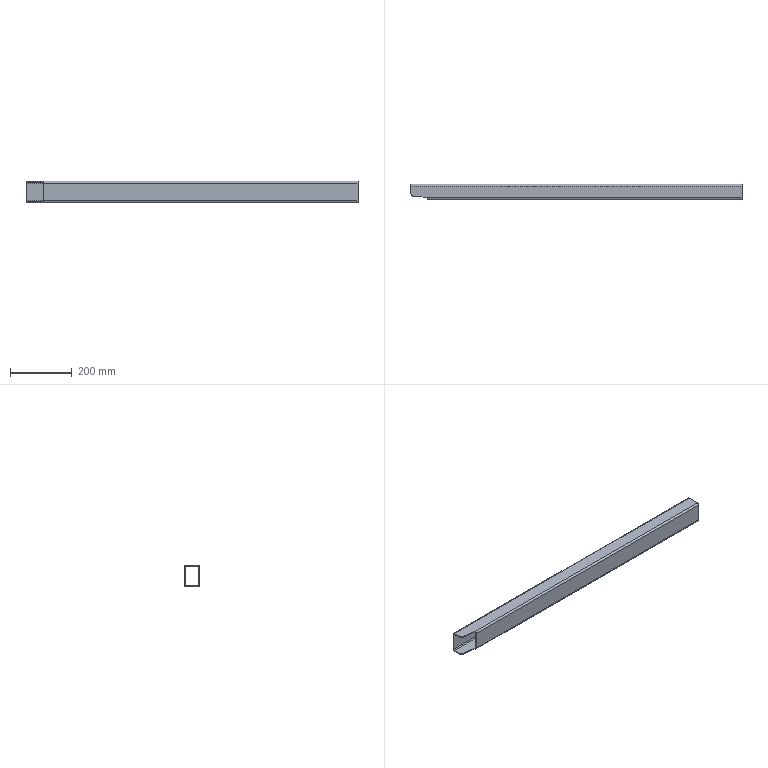Part | SolidWorks | 1 solid | 25 faces | box 1074 x 50 x 70 mm | volume 695582 mm3 | plane 17 | cylinder 8 | commonest cylinder face diameters 6 x4 12 x4
STEP:
#1=CARTESIAN_POINT('',(503.75,19.,35.));
#2=VERTEX_POINT('',#1);
#3=CARTESIAN_POINT('',(-569.75,19.,35.));
#4=VERTEX_POINT('',#3);
#5=CARTESIAN_POINT('',(569.75,19.,35.));
#6=DIRECTION('',(-1.,0.,0.));
#7=VECTOR('',#6,1000.);
#8=LINE('',#5,#7);
#9=EDGE_CURVE('',#2,#4,#8,.T.);
#10=ORIENTED_EDGE('',*,*,#9,.F.);
#11=CARTESIAN_POINT('',(503.75,25.,29.));
#12=VERTEX_POINT('',#11);
#13=CARTESIAN_POINT('',(503.75,19.,29.));
#14=DIRECTION('',(-1.,0.,0.));
#15=DIRECTION('',(0.,0.,1.));
#16=AXIS2_PLACEMENT_3D('',#13,#14,#15);
#17=CIRCLE('',#16,6.);
#18=EDGE_CURVE('',#2,#12,#17,.T.);
#19=ORIENTED_EDGE('',*,*,#18,.T.);
#20=CARTESIAN_POINT('',(-569.75,25.,29.));
#21=VERTEX_POINT('',#20);
#22=CARTESIAN_POINT('',(569.75,25.,29.));
#23=DIRECTION('',(-1.,0.,0.));
#24=VECTOR('',#23,1000.);
#25=LINE('',#22,#24);
#26=EDGE_CURVE('',#12,#21,#25,.T.);
#27=ORIENTED_EDGE('',*,*,#26,.T.);
#28=CARTESIAN_POINT('',(-569.75,19.,29.));
#29=DIRECTION('',(1.,0.,0.));
#30=DIRECTION('',(0.,1.,0.));
#31=AXIS2_PLACEMENT_3D('',#28,#29,#30);
#32=CIRCLE('',#31,6.);
#33=EDGE_CURVE('',#21,#4,#32,.T.);
#34=ORIENTED_EDGE('',*,*,#33,.T.);
#35=EDGE_LOOP('',(#10,#19,#27,#34));
#36=FACE_OUTER_BOUND('',#35,.T.);
#37=CARTESIAN_POINT('',(569.75,19.,29.));
#38=DIRECTION('',(-1.,0.,0.));
#39=DIRECTION('',(0.,-1.,0.));
#40=AXIS2_PLACEMENT_3D('',#37,#38,#39);
#41=CYLINDRICAL_SURFACE('',#40,6.);
#42=ADVANCED_FACE('',(#36),#41,.T.);
#43=CARTESIAN_POINT('',(503.75,-19.,35.));
#44=VERTEX_POINT('',#43);
#45=CARTESIAN_POINT('',(-513.25,-19.,35.));
#46=VERTEX_POINT('',#45);
#47=CARTESIAN_POINT('',(569.75,-19.,35.));
#48=DIRECTION('',(-1.,0.,0.));
#49=VECTOR('',#48,1000.);
#50=LINE('',#47,#49);
#51=EDGE_CURVE('',#44,#46,#50,.T.);
#52=ORIENTED_EDGE('',*,*,#51,.F.);
#53=CARTESIAN_POINT('',(503.75,30.,35.));
#54=DIRECTION('',(0.,-1.,0.));
#55=VECTOR('',#54,1000.);
#56=LINE('',#53,#55);
#57=EDGE_CURVE('',#2,#44,#56,.T.);
#58=ORIENTED_EDGE('',*,*,#57,.F.);
#59=ORIENTED_EDGE('',*,*,#9,.T.);
#60=CARTESIAN_POINT('',(-569.75,-3.027,35.));
#61=VERTEX_POINT('',#60);
#62=CARTESIAN_POINT('',(-569.75,19.,35.));
#63=DIRECTION('',(0.,-1.,0.));
#64=VECTOR('',#63,1000.);
#65=LINE('',#62,#64);
#66=EDGE_CURVE('',#4,#61,#65,.T.);
#67=ORIENTED_EDGE('',*,*,#66,.T.);
#68=CARTESIAN_POINT('',(-560.795,-12.972,35.));
#69=VERTEX_POINT('',#68);
#70=CARTESIAN_POINT('',(-560.795,-12.972,35.));
#71=DIRECTION('',(0.6691,-0.7431,0.));
#72=VECTOR('',#71,1000.);
#73=LINE('',#70,#72);
#74=EDGE_CURVE('',#61,#69,#73,.T.);
#75=ORIENTED_EDGE('',*,*,#74,.T.);
#76=CARTESIAN_POINT('',(-517.727,-17.499,35.));
#77=VERTEX_POINT('',#76);
#78=CARTESIAN_POINT('',(-517.727,-17.499,35.));
#79=DIRECTION('',(0.9945,-0.1045,0.));
#80=VECTOR('',#79,1000.);
#81=LINE('',#78,#80);
#82=EDGE_CURVE('',#69,#77,#81,.T.);
#83=ORIENTED_EDGE('',*,*,#82,.T.);
#84=CARTESIAN_POINT('',(-513.25,-19.,35.));
#85=DIRECTION('',(0.9481,-0.3179,0.));
#86=VECTOR('',#85,1000.);
#87=LINE('',#84,#86);
#88=EDGE_CURVE('',#77,#46,#87,.T.);
#89=ORIENTED_EDGE('',*,*,#88,.T.);
#90=EDGE_LOOP('',(#52,#58,#59,#67,#75,#83,#89));
#91=FACE_OUTER_BOUND('',#90,.T.);
#92=CARTESIAN_POINT('',(569.75,19.,35.));
#93=DIRECTION('',(0.,0.,-1.));
#94=DIRECTION('',(-1.,0.,0.));
#95=AXIS2_PLACEMENT_3D('',#92,#93,#94);
#96=PLANE('',#95);
#97=ADVANCED_FACE('',(#91),#96,.F.);
#98=CARTESIAN_POINT('',(503.75,-25.,29.));
#99=VERTEX_POINT('',#98);
#100=CARTESIAN_POINT('',(-513.25,-25.,29.));
#101=VERTEX_POINT('',#100);
#102=CARTESIAN_POINT('',(569.75,-25.,29.));
#103=DIRECTION('',(-1.,0.,0.));
#104=VECTOR('',#103,1000.);
#105=LINE('',#102,#104);
#106=EDGE_CURVE('',#99,#101,#105,.T.);
#107=ORIENTED_EDGE('',*,*,#106,.F.);
#108=CARTESIAN_POINT('',(503.75,-19.,29.));
#109=DIRECTION('',(-1.,0.,0.));
#110=DIRECTION('',(0.,0.,1.));
#111=AXIS2_PLACEMENT_3D('',#108,#109,#110);
#112=CIRCLE('',#111,6.);
#113=EDGE_CURVE('',#99,#44,#112,.T.);
#114=ORIENTED_EDGE('',*,*,#113,.T.);
#115=ORIENTED_EDGE('',*,*,#51,.T.);
#116=CARTESIAN_POINT('',(-513.25,-19.,29.));
#117=DIRECTION('',(1.,0.,0.));
#118=DIRECTION('',(0.,0.,-1.));
#119=AXIS2_PLACEMENT_3D('',#116,#117,#118);
#120=CIRCLE('',#119,6.);
#121=EDGE_CURVE('',#46,#101,#120,.T.);
#122=ORIENTED_EDGE('',*,*,#121,.T.);
#123=EDGE_LOOP('',(#107,#114,#115,#122));
#124=FACE_OUTER_BOUND('',#123,.T.);
#125=CARTESIAN_POINT('',(569.75,-19.,29.));
#126=DIRECTION('',(-1.,0.,0.));
#127=DIRECTION('',(0.,-1.,0.));
#128=AXIS2_PLACEMENT_3D('',#125,#126,#127);
#129=CYLINDRICAL_SURFACE('',#128,6.);
#130=ADVANCED_FACE('',(#124),#129,.T.);
#131=CARTESIAN_POINT('',(503.75,-25.,-29.));
#132=VERTEX_POINT('',#131);
#133=CARTESIAN_POINT('',(-513.25,-25.,-29.));
#134=VERTEX_POINT('',#133);
#135=CARTESIAN_POINT('',(569.75,-25.,-29.));
#136=DIRECTION('',(-1.,0.,0.));
#137=VECTOR('',#136,1000.);
#138=LINE('',#135,#137);
#139=EDGE_CURVE('',#132,#134,#138,.T.);
#140=ORIENTED_EDGE('',*,*,#139,.F.);
#141=CARTESIAN_POINT('',(503.75,-25.,-29.));
#142=DIRECTION('',(0.,0.,1.));
#143=VECTOR('',#142,1000.);
#144=LINE('',#141,#143);
#145=EDGE_CURVE('',#132,#99,#144,.T.);
#146=ORIENTED_EDGE('',*,*,#145,.T.);
#147=ORIENTED_EDGE('',*,*,#106,.T.);
#148=CARTESIAN_POINT('',(-513.25,-25.,-29.));
#149=DIRECTION('',(0.,0.,-1.));
#150=VECTOR('',#149,1000.);
#151=LINE('',#148,#150);
#152=EDGE_CURVE('',#101,#134,#151,.T.);
#153=ORIENTED_EDGE('',*,*,#152,.T.);
#154=EDGE_LOOP('',(#140,#146,#147,#153));
#155=FACE_OUTER_BOUND('',#154,.T.);
#156=CARTESIAN_POINT('',(569.75,-25.,-29.));
#157=DIRECTION('',(0.,1.,0.));
#158=DIRECTION('',(-1.,0.,0.));
#159=AXIS2_PLACEMENT_3D('',#156,#157,#158);
#160=PLANE('',#159);
#161=ADVANCED_FACE('',(#155),#160,.F.);
#162=CARTESIAN_POINT('',(503.75,-19.,-35.));
#163=VERTEX_POINT('',#162);
#164=CARTESIAN_POINT('',(-513.25,-19.,-35.));
#165=VERTEX_POINT('',#164);
#166=CARTESIAN_POINT('',(569.75,-19.,-35.));
#167=DIRECTION('',(-1.,0.,0.));
#168=VECTOR('',#167,1000.);
#169=LINE('',#166,#168);
#170=EDGE_CURVE('',#163,#165,#169,.T.);
#171=ORIENTED_EDGE('',*,*,#170,.F.);
#172=CARTESIAN_POINT('',(503.75,-19.,-29.));
#173=DIRECTION('',(-1.,0.,0.));
#174=DIRECTION('',(0.,0.,1.));
#175=AXIS2_PLACEMENT_3D('',#172,#173,#174);
#176=CIRCLE('',#175,6.);
#177=EDGE_CURVE('',#163,#132,#176,.T.);
#178=ORIENTED_EDGE('',*,*,#177,.T.);
#179=ORIENTED_EDGE('',*,*,#139,.T.);
#180=CARTESIAN_POINT('',(-513.25,-19.,-29.));
#181=DIRECTION('',(1.,0.,0.));
#182=DIRECTION('',(0.,0.,-1.));
#183=AXIS2_PLACEMENT_3D('',#180,#181,#182);
#184=CIRCLE('',#183,6.);
#185=EDGE_CURVE('',#134,#165,#184,.T.);
#186=ORIENTED_EDGE('',*,*,#185,.T.);
#187=EDGE_LOOP('',(#171,#178,#179,#186));
#188=FACE_OUTER_BOUND('',#187,.T.);
#189=CARTESIAN_POINT('',(569.75,-19.,-29.));
#190=DIRECTION('',(-1.,0.,0.));
#191=DIRECTION('',(0.,-1.,0.));
#192=AXIS2_PLACEMENT_3D('',#189,#190,#191);
#193=CYLINDRICAL_SURFACE('',#192,6.);
#194=ADVANCED_FACE('',(#188),#193,.T.);
#195=CARTESIAN_POINT('',(503.75,19.,-35.));
#196=VERTEX_POINT('',#195);
#197=CARTESIAN_POINT('',(-569.75,19.,-35.));
#198=VERTEX_POINT('',#197);
#199=CARTESIAN_POINT('',(569.75,19.,-35.));
#200=DIRECTION('',(-1.,0.,0.));
#201=VECTOR('',#200,1000.);
#202=LINE('',#199,#201);
#203=EDGE_CURVE('',#196,#198,#202,.T.);
#204=ORIENTED_EDGE('',*,*,#203,.F.);
#205=CARTESIAN_POINT('',(503.75,-19.,-35.));
#206=DIRECTION('',(0.,-1.,0.));
#207=VECTOR('',#206,1000.);
#208=LINE('',#205,#207);
#209=EDGE_CURVE('',#196,#163,#208,.T.);
#210=ORIENTED_EDGE('',*,*,#209,.T.);
#211=ORIENTED_EDGE('',*,*,#170,.T.);
#212=CARTESIAN_POINT('',(-517.727,-17.499,-35.));
#213=VERTEX_POINT('',#212);
#214=CARTESIAN_POINT('',(460.28,-345.454,-35.));
#215=DIRECTION('',(-0.9481,0.3179,0.));
#216=VECTOR('',#215,1000.);
#217=LINE('',#214,#216);
#218=EDGE_CURVE('',#165,#213,#217,.T.);
#219=ORIENTED_EDGE('',*,*,#218,.T.);
#220=CARTESIAN_POINT('',(-560.795,-12.972,-35.));
#221=VERTEX_POINT('',#220);
#222=CARTESIAN_POINT('',(558.024,-130.565,-35.));
#223=DIRECTION('',(-0.9945,0.1045,0.));
#224=VECTOR('',#223,1000.);
#225=LINE('',#222,#224);
#226=EDGE_CURVE('',#213,#221,#225,.T.);
#227=ORIENTED_EDGE('',*,*,#226,.T.);
#228=CARTESIAN_POINT('',(-569.75,-3.027,-35.));
#229=VERTEX_POINT('',#228);
#230=CARTESIAN_POINT('',(-51.612,-578.477,-35.));
#231=DIRECTION('',(-0.6691,0.7431,0.));
#232=VECTOR('',#231,1000.);
#233=LINE('',#230,#232);
#234=EDGE_CURVE('',#221,#229,#233,.T.);
#235=ORIENTED_EDGE('',*,*,#234,.T.);
#236=CARTESIAN_POINT('',(-569.75,-19.,-35.));
#237=DIRECTION('',(0.,1.,0.));
#238=VECTOR('',#237,1000.);
#239=LINE('',#236,#238);
#240=EDGE_CURVE('',#229,#198,#239,.T.);
#241=ORIENTED_EDGE('',*,*,#240,.T.);
#242=EDGE_LOOP('',(#204,#210,#211,#219,#227,#235,#241));
#243=FACE_OUTER_BOUND('',#242,.T.);
#244=CARTESIAN_POINT('',(569.75,-19.,-35.));
#245=DIRECTION('',(0.,0.,1.));
#246=DIRECTION('',(1.,0.,0.));
#247=AXIS2_PLACEMENT_3D('',#244,#245,#246);
#248=PLANE('',#247);
#249=ADVANCED_FACE('',(#243),#248,.F.);
#250=CARTESIAN_POINT('',(503.75,25.,-29.));
#251=VERTEX_POINT('',#250);
#252=CARTESIAN_POINT('',(-569.75,25.,-29.));
#253=VERTEX_POINT('',#252);
#254=CARTESIAN_POINT('',(569.75,25.,-29.));
#255=DIRECTION('',(-1.,0.,0.));
#256=VECTOR('',#255,1000.);
#257=LINE('',#254,#256);
#258=EDGE_CURVE('',#251,#253,#257,.T.);
#259=ORIENTED_EDGE('',*,*,#258,.F.);
#260=CARTESIAN_POINT('',(503.75,19.,-29.));
#261=DIRECTION('',(-1.,0.,0.));
#262=DIRECTION('',(0.,0.,1.));
#263=AXIS2_PLACEMENT_3D('',#260,#261,#262);
#264=CIRCLE('',#263,6.);
#265=EDGE_CURVE('',#251,#196,#264,.T.);
#266=ORIENTED_EDGE('',*,*,#265,.T.);
#267=ORIENTED_EDGE('',*,*,#203,.T.);
#268=CARTESIAN_POINT('',(-569.75,19.,-29.));
#269=DIRECTION('',(1.,0.,0.));
#270=DIRECTION('',(0.,1.,0.));
#271=AXIS2_PLACEMENT_3D('',#268,#269,#270);
#272=CIRCLE('',#271,6.);
#273=EDGE_CURVE('',#198,#253,#272,.T.);
#274=ORIENTED_EDGE('',*,*,#273,.T.);
#275=EDGE_LOOP('',(#259,#266,#267,#274));
#276=FACE_OUTER_BOUND('',#275,.T.);
#277=CARTESIAN_POINT('',(569.75,19.,-29.));
#278=DIRECTION('',(-1.,0.,0.));
#279=DIRECTION('',(0.,-1.,0.));
#280=AXIS2_PLACEMENT_3D('',#277,#278,#279);
#281=CYLINDRICAL_SURFACE('',#280,6.);
#282=ADVANCED_FACE('',(#276),#281,.T.);
#283=CARTESIAN_POINT('',(503.75,-22.,29.));
#284=VERTEX_POINT('',#283);
#285=CARTESIAN_POINT('',(503.75,-19.,32.));
#286=VERTEX_POINT('',#285);
#287=CARTESIAN_POINT('',(503.75,-19.,29.));
#288=DIRECTION('',(-1.,0.,0.));
#289=DIRECTION('',(0.,0.,1.));
#290=AXIS2_PLACEMENT_3D('',#287,#288,#289);
#291=CIRCLE('',#290,3.);
#292=EDGE_CURVE('',#284,#286,#291,.T.);
#293=ORIENTED_EDGE('',*,*,#292,.F.);
#294=CARTESIAN_POINT('',(-513.25,-22.,29.));
#295=VERTEX_POINT('',#294);
#296=CARTESIAN_POINT('',(569.75,-22.,29.));
#297=DIRECTION('',(-1.,0.,0.));
#298=VECTOR('',#297,1000.);
#299=LINE('',#296,#298);
#300=EDGE_CURVE('',#284,#295,#299,.T.);
#301=ORIENTED_EDGE('',*,*,#300,.T.);
#302=CARTESIAN_POINT('',(-513.25,-19.,32.));
#303=VERTEX_POINT('',#302);
#304=CARTESIAN_POINT('',(-513.25,-19.,29.));
#305=DIRECTION('',(1.,0.,0.));
#306=DIRECTION('',(0.,0.,-1.));
#307=AXIS2_PLACEMENT_3D('',#304,#305,#306);
#308=CIRCLE('',#307,3.);
#309=EDGE_CURVE('',#303,#295,#308,.T.);
#310=ORIENTED_EDGE('',*,*,#309,.F.);
#311=CARTESIAN_POINT('',(569.75,-19.,32.));
#312=DIRECTION('',(-1.,0.,0.));
#313=VECTOR('',#312,1000.);
#314=LINE('',#311,#313);
#315=EDGE_CURVE('',#286,#303,#314,.T.);
#316=ORIENTED_EDGE('',*,*,#315,.F.);
#317=EDGE_LOOP('',(#293,#301,#310,#316));
#318=FACE_OUTER_BOUND('',#317,.T.);
#319=CARTESIAN_POINT('',(569.75,-19.,29.));
#320=DIRECTION('',(-1.,0.,0.));
#321=DIRECTION('',(0.,-1.,0.));
#322=AXIS2_PLACEMENT_3D('',#319,#320,#321);
#323=CYLINDRICAL_SURFACE('',#322,3.);
#324=ADVANCED_FACE('',(#318),#323,.F.);
#325=CARTESIAN_POINT('',(503.75,19.,32.));
#326=VERTEX_POINT('',#325);
#327=CARTESIAN_POINT('',(503.75,19.,32.));
#328=DIRECTION('',(0.,1.,0.));
#329=VECTOR('',#328,1000.);
#330=LINE('',#327,#329);
#331=EDGE_CURVE('',#286,#326,#330,.T.);
#332=ORIENTED_EDGE('',*,*,#331,.F.);
#333=ORIENTED_EDGE('',*,*,#315,.T.);
#334=CARTESIAN_POINT('',(-517.727,-17.499,32.));
#335=VERTEX_POINT('',#334);
#336=CARTESIAN_POINT('',(448.825,-341.613,32.));
#337=DIRECTION('',(0.9481,-0.3179,0.));
#338=VECTOR('',#337,1000.);
#339=LINE('',#336,#338);
#340=EDGE_CURVE('',#335,#303,#339,.T.);
#341=ORIENTED_EDGE('',*,*,#340,.F.);
#342=CARTESIAN_POINT('',(-560.795,-12.972,32.));
#343=VERTEX_POINT('',#342);
#344=CARTESIAN_POINT('',(554.074,-130.149,32.));
#345=DIRECTION('',(0.9945,-0.1045,0.));
#346=VECTOR('',#345,1000.);
#347=LINE('',#344,#346);
#348=EDGE_CURVE('',#343,#335,#347,.T.);
#349=ORIENTED_EDGE('',*,*,#348,.F.);
#350=CARTESIAN_POINT('',(-569.75,-3.027,32.));
#351=VERTEX_POINT('',#350);
#352=CARTESIAN_POINT('',(-70.508,-557.491,32.));
#353=DIRECTION('',(0.6691,-0.7431,0.));
#354=VECTOR('',#353,1000.);
#355=LINE('',#352,#354);
#356=EDGE_CURVE('',#351,#343,#355,.T.);
#357=ORIENTED_EDGE('',*,*,#356,.F.);
#358=CARTESIAN_POINT('',(-569.75,19.,32.));
#359=VERTEX_POINT('',#358);
#360=CARTESIAN_POINT('',(-569.75,19.,32.));
#361=DIRECTION('',(0.,-1.,0.));
#362=VECTOR('',#361,1000.);
#363=LINE('',#360,#362);
#364=EDGE_CURVE('',#359,#351,#363,.T.);
#365=ORIENTED_EDGE('',*,*,#364,.F.);
#366=CARTESIAN_POINT('',(569.75,19.,32.));
#367=DIRECTION('',(-1.,0.,0.));
#368=VECTOR('',#367,1000.);
#369=LINE('',#366,#368);
#370=EDGE_CURVE('',#326,#359,#369,.T.);
#371=ORIENTED_EDGE('',*,*,#370,.F.);
#372=EDGE_LOOP('',(#332,#333,#341,#349,#357,#365,#371));
#373=FACE_OUTER_BOUND('',#372,.T.);
#374=CARTESIAN_POINT('',(569.75,19.,32.));
#375=DIRECTION('',(0.,0.,-1.));
#376=DIRECTION('',(-1.,0.,0.));
#377=AXIS2_PLACEMENT_3D('',#374,#375,#376);
#378=PLANE('',#377);
#379=ADVANCED_FACE('',(#373),#378,.T.);
#380=CARTESIAN_POINT('',(503.75,22.,29.));
#381=VERTEX_POINT('',#380);
#382=CARTESIAN_POINT('',(503.75,19.,29.));
#383=DIRECTION('',(-1.,0.,0.));
#384=DIRECTION('',(0.,0.,1.));
#385=AXIS2_PLACEMENT_3D('',#382,#383,#384);
#386=CIRCLE('',#385,3.);
#387=EDGE_CURVE('',#326,#381,#386,.T.);
#388=ORIENTED_EDGE('',*,*,#387,.F.);
#389=ORIENTED_EDGE('',*,*,#370,.T.);
#390=CARTESIAN_POINT('',(-569.75,22.,29.));
#391=VERTEX_POINT('',#390);
#392=CARTESIAN_POINT('',(-569.75,19.,29.));
#393=DIRECTION('',(1.,0.,0.));
#394=DIRECTION('',(0.,1.,0.));
#395=AXIS2_PLACEMENT_3D('',#392,#393,#394);
#396=CIRCLE('',#395,3.);
#397=EDGE_CURVE('',#391,#359,#396,.T.);
#398=ORIENTED_EDGE('',*,*,#397,.F.);
#399=CARTESIAN_POINT('',(569.75,22.,29.));
#400=DIRECTION('',(-1.,0.,0.));
#401=VECTOR('',#400,1000.);
#402=LINE('',#399,#401);
#403=EDGE_CURVE('',#381,#391,#402,.T.);
#404=ORIENTED_EDGE('',*,*,#403,.F.);
#405=EDGE_LOOP('',(#388,#389,#398,#404));
#406=FACE_OUTER_BOUND('',#405,.T.);
#407=CARTESIAN_POINT('',(569.75,19.,29.));
#408=DIRECTION('',(-1.,0.,0.));
#409=DIRECTION('',(0.,-1.,0.));
#410=AXIS2_PLACEMENT_3D('',#407,#408,#409);
#411=CYLINDRICAL_SURFACE('',#410,3.);
#412=ADVANCED_FACE('',(#406),#411,.F.);
#413=CARTESIAN_POINT('',(503.75,22.,-29.));
#414=VERTEX_POINT('',#413);
#415=CARTESIAN_POINT('',(503.75,22.,29.));
#416=DIRECTION('',(0.,0.,-1.));
#417=VECTOR('',#416,1000.);
#418=LINE('',#415,#417);
#419=EDGE_CURVE('',#381,#414,#418,.T.);
#420=ORIENTED_EDGE('',*,*,#419,.F.);
#421=ORIENTED_EDGE('',*,*,#403,.T.);
#422=CARTESIAN_POINT('',(-569.75,22.,-29.));
#423=VERTEX_POINT('',#422);
#424=CARTESIAN_POINT('',(-569.75,22.,29.));
#425=DIRECTION('',(0.,0.,1.));
#426=VECTOR('',#425,1000.);
#427=LINE('',#424,#426);
#428=EDGE_CURVE('',#423,#391,#427,.T.);
#429=ORIENTED_EDGE('',*,*,#428,.F.);
#430=CARTESIAN_POINT('',(569.75,22.,-29.));
#431=DIRECTION('',(-1.,0.,0.));
#432=VECTOR('',#431,1000.);
#433=LINE('',#430,#432);
#434=EDGE_CURVE('',#414,#423,#433,.T.);
#435=ORIENTED_EDGE('',*,*,#434,.F.);
#436=EDGE_LOOP('',(#420,#421,#429,#435));
#437=FACE_OUTER_BOUND('',#436,.T.);
#438=CARTESIAN_POINT('',(569.75,22.,29.));
#439=DIRECTION('',(0.,-1.,0.));
#440=DIRECTION('',(1.,0.,0.));
#441=AXIS2_PLACEMENT_3D('',#438,#439,#440);
#442=PLANE('',#441);
#443=ADVANCED_FACE('',(#437),#442,.T.);
#444=CARTESIAN_POINT('',(503.75,19.,-32.));
#445=VERTEX_POINT('',#444);
#446=CARTESIAN_POINT('',(503.75,19.,-29.));
#447=DIRECTION('',(-1.,0.,0.));
#448=DIRECTION('',(0.,0.,1.));
#449=AXIS2_PLACEMENT_3D('',#446,#447,#448);
#450=CIRCLE('',#449,3.);
#451=EDGE_CURVE('',#414,#445,#450,.T.);
#452=ORIENTED_EDGE('',*,*,#451,.F.);
#453=ORIENTED_EDGE('',*,*,#434,.T.);
#454=CARTESIAN_POINT('',(-569.75,19.,-32.));
#455=VERTEX_POINT('',#454);
#456=CARTESIAN_POINT('',(-569.75,19.,-29.));
#457=DIRECTION('',(1.,0.,0.));
#458=DIRECTION('',(0.,1.,0.));
#459=AXIS2_PLACEMENT_3D('',#456,#457,#458);
#460=CIRCLE('',#459,3.);
#461=EDGE_CURVE('',#455,#423,#460,.T.);
#462=ORIENTED_EDGE('',*,*,#461,.F.);
#463=CARTESIAN_POINT('',(569.75,19.,-32.));
#464=DIRECTION('',(-1.,0.,0.));
#465=VECTOR('',#464,1000.);
#466=LINE('',#463,#465);
#467=EDGE_CURVE('',#445,#455,#466,.T.);
#468=ORIENTED_EDGE('',*,*,#467,.F.);
#469=EDGE_LOOP('',(#452,#453,#462,#468));
#470=FACE_OUTER_BOUND('',#469,.T.);
#471=CARTESIAN_POINT('',(569.75,19.,-29.));
#472=DIRECTION('',(-1.,0.,0.));
#473=DIRECTION('',(0.,-1.,0.));
#474=AXIS2_PLACEMENT_3D('',#471,#472,#473);
#475=CYLINDRICAL_SURFACE('',#474,3.);
#476=ADVANCED_FACE('',(#470),#475,.F.);
#477=CARTESIAN_POINT('',(503.75,-19.,-32.));
#478=VERTEX_POINT('',#477);
#479=CARTESIAN_POINT('',(503.75,-19.,-32.));
#480=DIRECTION('',(0.,-1.,0.));
#481=VECTOR('',#480,1000.);
#482=LINE('',#479,#481);
#483=EDGE_CURVE('',#445,#478,#482,.T.);
#484=ORIENTED_EDGE('',*,*,#483,.F.);
#485=ORIENTED_EDGE('',*,*,#467,.T.);
#486=CARTESIAN_POINT('',(-569.75,-3.027,-32.));
#487=VERTEX_POINT('',#486);
#488=CARTESIAN_POINT('',(-569.75,-19.,-32.));
#489=DIRECTION('',(0.,1.,0.));
#490=VECTOR('',#489,1000.);
#491=LINE('',#488,#490);
#492=EDGE_CURVE('',#487,#455,#491,.T.);
#493=ORIENTED_EDGE('',*,*,#492,.F.);
#494=CARTESIAN_POINT('',(-560.795,-12.972,-32.));
#495=VERTEX_POINT('',#494);
#496=CARTESIAN_POINT('',(-51.612,-578.477,-32.));
#497=DIRECTION('',(-0.6691,0.7431,0.));
#498=VECTOR('',#497,1000.);
#499=LINE('',#496,#498);
#500=EDGE_CURVE('',#495,#487,#499,.T.);
#501=ORIENTED_EDGE('',*,*,#500,.F.);
#502=CARTESIAN_POINT('',(-517.727,-17.499,-32.));
#503=VERTEX_POINT('',#502);
#504=CARTESIAN_POINT('',(558.024,-130.565,-32.));
#505=DIRECTION('',(-0.9945,0.1045,0.));
#506=VECTOR('',#505,1000.);
#507=LINE('',#504,#506);
#508=EDGE_CURVE('',#503,#495,#507,.T.);
#509=ORIENTED_EDGE('',*,*,#508,.F.);
#510=CARTESIAN_POINT('',(-513.25,-19.,-32.));
#511=VERTEX_POINT('',#510);
#512=CARTESIAN_POINT('',(460.28,-345.454,-32.));
#513=DIRECTION('',(-0.9481,0.3179,0.));
#514=VECTOR('',#513,1000.);
#515=LINE('',#512,#514);
#516=EDGE_CURVE('',#511,#503,#515,.T.);
#517=ORIENTED_EDGE('',*,*,#516,.F.);
#518=CARTESIAN_POINT('',(569.75,-19.,-32.));
#519=DIRECTION('',(-1.,0.,0.));
#520=VECTOR('',#519,1000.);
#521=LINE('',#518,#520);
#522=EDGE_CURVE('',#478,#511,#521,.T.);
#523=ORIENTED_EDGE('',*,*,#522,.F.);
#524=EDGE_LOOP('',(#484,#485,#493,#501,#509,#517,#523));
#525=FACE_OUTER_BOUND('',#524,.T.);
#526=CARTESIAN_POINT('',(569.75,-19.,-32.));
#527=DIRECTION('',(0.,0.,1.));
#528=DIRECTION('',(1.,0.,0.));
#529=AXIS2_PLACEMENT_3D('',#526,#527,#528);
#530=PLANE('',#529);
#531=ADVANCED_FACE('',(#525),#530,.T.);
#532=CARTESIAN_POINT('',(503.75,-22.,-29.));
#533=VERTEX_POINT('',#532);
#534=CARTESIAN_POINT('',(503.75,-19.,-29.));
#535=DIRECTION('',(-1.,0.,0.));
#536=DIRECTION('',(0.,0.,1.));
#537=AXIS2_PLACEMENT_3D('',#534,#535,#536);
#538=CIRCLE('',#537,3.);
#539=EDGE_CURVE('',#478,#533,#538,.T.);
#540=ORIENTED_EDGE('',*,*,#539,.F.);
#541=ORIENTED_EDGE('',*,*,#522,.T.);
#542=CARTESIAN_POINT('',(-513.25,-22.,-29.));
#543=VERTEX_POINT('',#542);
#544=CARTESIAN_POINT('',(-513.25,-19.,-29.));
#545=DIRECTION('',(1.,0.,0.));
#546=DIRECTION('',(0.,0.,-1.));
#547=AXIS2_PLACEMENT_3D('',#544,#545,#546);
#548=CIRCLE('',#547,3.);
#549=EDGE_CURVE('',#543,#511,#548,.T.);
#550=ORIENTED_EDGE('',*,*,#549,.F.);
#551=CARTESIAN_POINT('',(569.75,-22.,-29.));
#552=DIRECTION('',(-1.,0.,0.));
#553=VECTOR('',#552,1000.);
#554=LINE('',#551,#553);
#555=EDGE_CURVE('',#533,#543,#554,.T.);
#556=ORIENTED_EDGE('',*,*,#555,.F.);
#557=EDGE_LOOP('',(#540,#541,#550,#556));
#558=FACE_OUTER_BOUND('',#557,.T.);
#559=CARTESIAN_POINT('',(569.75,-19.,-29.));
#560=DIRECTION('',(-1.,0.,0.));
#561=DIRECTION('',(0.,-1.,0.));
#562=AXIS2_PLACEMENT_3D('',#559,#560,#561);
#563=CYLINDRICAL_SURFACE('',#562,3.);
#564=ADVANCED_FACE('',(#558),#563,.F.);
#565=CARTESIAN_POINT('',(503.75,-22.,-29.));
#566=DIRECTION('',(0.,0.,1.));
#567=VECTOR('',#566,1000.);
#568=LINE('',#565,#567);
#569=EDGE_CURVE('',#533,#284,#568,.T.);
#570=ORIENTED_EDGE('',*,*,#569,.F.);
#571=ORIENTED_EDGE('',*,*,#555,.T.);
#572=CARTESIAN_POINT('',(-513.25,-22.,-29.));
#573=DIRECTION('',(0.,0.,-1.));
#574=VECTOR('',#573,1000.);
#575=LINE('',#572,#574);
#576=EDGE_CURVE('',#295,#543,#575,.T.);
#577=ORIENTED_EDGE('',*,*,#576,.F.);
#578=ORIENTED_EDGE('',*,*,#300,.F.);
#579=EDGE_LOOP('',(#570,#571,#577,#578));
#580=FACE_OUTER_BOUND('',#579,.T.);
#581=CARTESIAN_POINT('',(569.75,-22.,-29.));
#582=DIRECTION('',(0.,1.,0.));
#583=DIRECTION('',(-1.,0.,0.));
#584=AXIS2_PLACEMENT_3D('',#581,#582,#583);
#585=PLANE('',#584);
#586=ADVANCED_FACE('',(#580),#585,.T.);
#587=ORIENTED_EDGE('',*,*,#26,.F.);
#588=CARTESIAN_POINT('',(503.75,25.,29.));
#589=DIRECTION('',(0.,0.,-1.));
#590=VECTOR('',#589,1000.);
#591=LINE('',#588,#590);
#592=EDGE_CURVE('',#12,#251,#591,.T.);
#593=ORIENTED_EDGE('',*,*,#592,.T.);
#594=ORIENTED_EDGE('',*,*,#258,.T.);
#595=CARTESIAN_POINT('',(-569.75,25.,29.));
#596=DIRECTION('',(0.,0.,1.));
#597=VECTOR('',#596,1000.);
#598=LINE('',#595,#597);
#599=EDGE_CURVE('',#253,#21,#598,.T.);
#600=ORIENTED_EDGE('',*,*,#599,.T.);
#601=EDGE_LOOP('',(#587,#593,#594,#600));
#602=FACE_OUTER_BOUND('',#601,.T.);
#603=CARTESIAN_POINT('',(569.75,25.,29.));
#604=DIRECTION('',(0.,-1.,0.));
#605=DIRECTION('',(1.,0.,0.));
#606=AXIS2_PLACEMENT_3D('',#603,#604,#605);
#607=PLANE('',#606);
#608=ADVANCED_FACE('',(#602),#607,.F.);
#609=ORIENTED_EDGE('',*,*,#240,.F.);
#610=CARTESIAN_POINT('',(-569.75,-3.027,29.));
#611=DIRECTION('',(0.,0.,1.));
#612=VECTOR('',#611,1000.);
#613=LINE('',#610,#612);
#614=EDGE_CURVE('',#229,#487,#613,.T.);
#615=ORIENTED_EDGE('',*,*,#614,.T.);
#616=ORIENTED_EDGE('',*,*,#492,.T.);
#617=ORIENTED_EDGE('',*,*,#461,.T.);
#618=ORIENTED_EDGE('',*,*,#428,.T.);
#619=ORIENTED_EDGE('',*,*,#397,.T.);
#620=ORIENTED_EDGE('',*,*,#364,.T.);
#621=CARTESIAN_POINT('',(-569.75,-3.027,35.));
#622=DIRECTION('',(0.,0.,-1.));
#623=VECTOR('',#622,1000.);
#624=LINE('',#621,#623);
#625=EDGE_CURVE('',#61,#351,#624,.T.);
#626=ORIENTED_EDGE('',*,*,#625,.F.);
#627=ORIENTED_EDGE('',*,*,#66,.F.);
#628=ORIENTED_EDGE('',*,*,#33,.F.);
#629=ORIENTED_EDGE('',*,*,#599,.F.);
#630=ORIENTED_EDGE('',*,*,#273,.F.);
#631=EDGE_LOOP('',(#609,#615,#616,#617,#618,#619,#620,#626,#627,#628,#629,#630));
#632=FACE_OUTER_BOUND('',#631,.T.);
#633=CARTESIAN_POINT('',(-569.75,19.,29.));
#634=DIRECTION('',(1.,0.,0.));
#635=DIRECTION('',(0.,1.,0.));
#636=AXIS2_PLACEMENT_3D('',#633,#634,#635);
#637=PLANE('',#636);
#638=ADVANCED_FACE('',(#632),#637,.F.);
#639=CARTESIAN_POINT('',(-517.727,-17.499,35.));
#640=DIRECTION('',(0.,0.,-1.));
#641=VECTOR('',#640,1000.);
#642=LINE('',#639,#641);
#643=EDGE_CURVE('',#503,#213,#642,.T.);
#644=ORIENTED_EDGE('',*,*,#643,.F.);
#645=ORIENTED_EDGE('',*,*,#508,.T.);
#646=CARTESIAN_POINT('',(-560.795,-12.972,35.));
#647=DIRECTION('',(0.,0.,-1.));
#648=VECTOR('',#647,1000.);
#649=LINE('',#646,#648);
#650=EDGE_CURVE('',#495,#221,#649,.T.);
#651=ORIENTED_EDGE('',*,*,#650,.T.);
#652=ORIENTED_EDGE('',*,*,#226,.F.);
#653=EDGE_LOOP('',(#644,#645,#651,#652));
#654=FACE_OUTER_BOUND('',#653,.T.);
#655=CARTESIAN_POINT('',(-517.727,-17.499,35.));
#656=DIRECTION('',(0.1045,0.9945,0.));
#657=DIRECTION('',(-0.9945,0.1045,0.));
#658=AXIS2_PLACEMENT_3D('',#655,#656,#657);
#659=PLANE('',#658);
#660=ADVANCED_FACE('',(#654),#659,.F.);
#661=ORIENTED_EDGE('',*,*,#348,.T.);
#662=CARTESIAN_POINT('',(-517.727,-17.499,35.));
#663=DIRECTION('',(0.,0.,-1.));
#664=VECTOR('',#663,1000.);
#665=LINE('',#662,#664);
#666=EDGE_CURVE('',#77,#335,#665,.T.);
#667=ORIENTED_EDGE('',*,*,#666,.F.);
#668=ORIENTED_EDGE('',*,*,#82,.F.);
#669=CARTESIAN_POINT('',(-560.795,-12.972,35.));
#670=DIRECTION('',(0.,0.,-1.));
#671=VECTOR('',#670,1000.);
#672=LINE('',#669,#671);
#673=EDGE_CURVE('',#69,#343,#672,.T.);
#674=ORIENTED_EDGE('',*,*,#673,.T.);
#675=EDGE_LOOP('',(#661,#667,#668,#674));
#676=FACE_OUTER_BOUND('',#675,.T.);
#677=CARTESIAN_POINT('',(-517.727,-17.499,35.));
#678=DIRECTION('',(0.1045,0.9945,0.));
#679=DIRECTION('',(-0.9945,0.1045,0.));
#680=AXIS2_PLACEMENT_3D('',#677,#678,#679);
#681=PLANE('',#680);
#682=ADVANCED_FACE('',(#676),#681,.F.);
#683=CARTESIAN_POINT('',(-513.25,-19.,35.));
#684=DIRECTION('',(0.,0.,-1.));
#685=VECTOR('',#684,1000.);
#686=LINE('',#683,#685);
#687=EDGE_CURVE('',#511,#165,#686,.T.);
#688=ORIENTED_EDGE('',*,*,#687,.F.);
#689=ORIENTED_EDGE('',*,*,#516,.T.);
#690=ORIENTED_EDGE('',*,*,#643,.T.);
#691=ORIENTED_EDGE('',*,*,#218,.F.);
#692=EDGE_LOOP('',(#688,#689,#690,#691));
#693=FACE_OUTER_BOUND('',#692,.T.);
#694=CARTESIAN_POINT('',(-513.25,-19.,35.));
#695=DIRECTION('',(0.3179,0.9481,0.));
#696=DIRECTION('',(-0.9481,0.3179,0.));
#697=AXIS2_PLACEMENT_3D('',#694,#695,#696);
#698=PLANE('',#697);
#699=ADVANCED_FACE('',(#693),#698,.F.);
#700=ORIENTED_EDGE('',*,*,#340,.T.);
#701=CARTESIAN_POINT('',(-513.25,-19.,35.));
#702=DIRECTION('',(0.,0.,-1.));
#703=VECTOR('',#702,1000.);
#704=LINE('',#701,#703);
#705=EDGE_CURVE('',#46,#303,#704,.T.);
#706=ORIENTED_EDGE('',*,*,#705,.F.);
#707=ORIENTED_EDGE('',*,*,#88,.F.);
#708=ORIENTED_EDGE('',*,*,#666,.T.);
#709=EDGE_LOOP('',(#700,#706,#707,#708));
#710=FACE_OUTER_BOUND('',#709,.T.);
#711=CARTESIAN_POINT('',(-513.25,-19.,35.));
#712=DIRECTION('',(0.3179,0.9481,0.));
#713=DIRECTION('',(-0.9481,0.3179,0.));
#714=AXIS2_PLACEMENT_3D('',#711,#712,#713);
#715=PLANE('',#714);
#716=ADVANCED_FACE('',(#710),#715,.F.);
#717=ORIENTED_EDGE('',*,*,#705,.T.);
#718=ORIENTED_EDGE('',*,*,#309,.T.);
#719=ORIENTED_EDGE('',*,*,#576,.T.);
#720=ORIENTED_EDGE('',*,*,#549,.T.);
#721=ORIENTED_EDGE('',*,*,#687,.T.);
#722=ORIENTED_EDGE('',*,*,#185,.F.);
#723=ORIENTED_EDGE('',*,*,#152,.F.);
#724=ORIENTED_EDGE('',*,*,#121,.F.);
#725=EDGE_LOOP('',(#717,#718,#719,#720,#721,#722,#723,#724));
#726=FACE_OUTER_BOUND('',#725,.T.);
#727=CARTESIAN_POINT('',(-513.25,-25.,35.));
#728=DIRECTION('',(1.,0.,0.));
#729=DIRECTION('',(0.,0.,-1.));
#730=AXIS2_PLACEMENT_3D('',#727,#728,#729);
#731=PLANE('',#730);
#732=ADVANCED_FACE('',(#726),#731,.F.);
#733=ORIENTED_EDGE('',*,*,#650,.F.);
#734=ORIENTED_EDGE('',*,*,#500,.T.);
#735=ORIENTED_EDGE('',*,*,#614,.F.);
#736=ORIENTED_EDGE('',*,*,#234,.F.);
#737=EDGE_LOOP('',(#733,#734,#735,#736));
#738=FACE_OUTER_BOUND('',#737,.T.);
#739=CARTESIAN_POINT('',(-560.795,-12.972,35.));
#740=DIRECTION('',(0.7431,0.6691,0.));
#741=DIRECTION('',(-0.6691,0.7431,0.));
#742=AXIS2_PLACEMENT_3D('',#739,#740,#741);
#743=PLANE('',#742);
#744=ADVANCED_FACE('',(#738),#743,.F.);
#745=ORIENTED_EDGE('',*,*,#356,.T.);
#746=ORIENTED_EDGE('',*,*,#673,.F.);
#747=ORIENTED_EDGE('',*,*,#74,.F.);
#748=ORIENTED_EDGE('',*,*,#625,.T.);
#749=EDGE_LOOP('',(#745,#746,#747,#748));
#750=FACE_OUTER_BOUND('',#749,.T.);
#751=CARTESIAN_POINT('',(-560.795,-12.972,35.));
#752=DIRECTION('',(0.7431,0.6691,0.));
#753=DIRECTION('',(-0.6691,0.7431,0.));
#754=AXIS2_PLACEMENT_3D('',#751,#752,#753);
#755=PLANE('',#754);
#756=ADVANCED_FACE('',(#750),#755,.F.);
#757=ORIENTED_EDGE('',*,*,#292,.T.);
#758=ORIENTED_EDGE('',*,*,#331,.T.);
#759=ORIENTED_EDGE('',*,*,#387,.T.);
#760=ORIENTED_EDGE('',*,*,#419,.T.);
#761=ORIENTED_EDGE('',*,*,#451,.T.);
#762=ORIENTED_EDGE('',*,*,#483,.T.);
#763=ORIENTED_EDGE('',*,*,#539,.T.);
#764=ORIENTED_EDGE('',*,*,#569,.T.);
#765=EDGE_LOOP('',(#757,#758,#759,#760,#761,#762,#763,#764));
#766=FACE_BOUND('',#765,.T.);
#767=ORIENTED_EDGE('',*,*,#57,.T.);
#768=ORIENTED_EDGE('',*,*,#113,.F.);
#769=ORIENTED_EDGE('',*,*,#145,.F.);
#770=ORIENTED_EDGE('',*,*,#177,.F.);
#771=ORIENTED_EDGE('',*,*,#209,.F.);
#772=ORIENTED_EDGE('',*,*,#265,.F.);
#773=ORIENTED_EDGE('',*,*,#592,.F.);
#774=ORIENTED_EDGE('',*,*,#18,.F.);
#775=EDGE_LOOP('',(#767,#768,#769,#770,#771,#772,#773,#774));
#776=FACE_OUTER_BOUND('',#775,.T.);
#777=CARTESIAN_POINT('',(503.75,30.,-35.));
#778=DIRECTION('',(-1.,0.,0.));
#779=DIRECTION('',(0.,0.,1.));
#780=AXIS2_PLACEMENT_3D('',#777,#778,#779);
#781=PLANE('',#780);
#782=ADVANCED_FACE('',(#766,#776),#781,.F.);
#783=CLOSED_SHELL('',(#42,#97,#130,#161,#194,#249,#282,#324,#379,#412,#443,#476,#531,#564,#586,#608,#638,#660,#682,#699,#716,#732,#744,#756,#782));
#784=MANIFOLD_SOLID_BREP('',#783);
#785=CARTESIAN_POINT('',(0.,0.,0.));
#786=DIRECTION('',(0.,0.,1.));
#787=DIRECTION('',(1.,0.,0.));
#788=AXIS2_PLACEMENT_3D('',#785,#786,#787);
#789=(LENGTH_UNIT()NAMED_UNIT(*)SI_UNIT(.MILLI.,.METRE.));
#790=UNCERTAINTY_MEASURE_WITH_UNIT(LENGTH_MEASURE(0.00001),#789,'','');
#791=(NAMED_UNIT(*)PLANE_ANGLE_UNIT()SI_UNIT($,.RADIAN.));
#792=(NAMED_UNIT(*)SI_UNIT($,.STERADIAN.)SOLID_ANGLE_UNIT());
#793=(GEOMETRIC_REPRESENTATION_CONTEXT(3)GLOBAL_UNCERTAINTY_ASSIGNED_CONTEXT((#790))GLOBAL_UNIT_ASSIGNED_CONTEXT((#789,#791,#792))REPRESENTATION_CONTEXT('',''));
#794=ADVANCED_BREP_SHAPE_REPRESENTATION('',(#784,#788),#793);